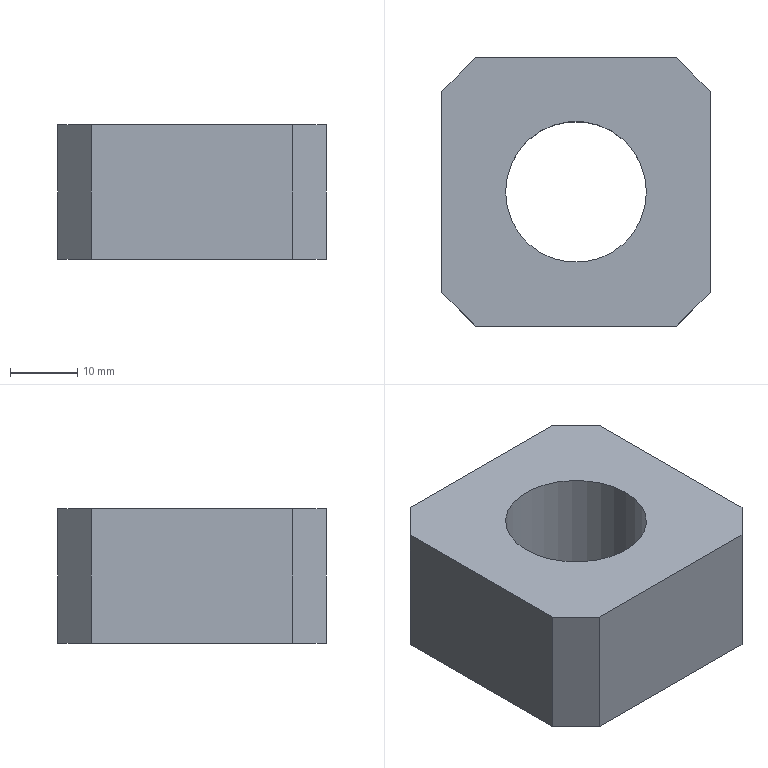CAM job | NX | 3-axis milling, drilling | part box 40 x 40 x 20 mm | stock box 45 x 45 x 25 mm
Tools:
number,name,description,diameter,corner_radius,flute_length,length,flutes
5,D10开粗,D10,10.0,0.0,25.0,75.0,2
7,D10精光,D10,10.0,0.0,25.0,75.0,2
2,D8倒角刀,DJ8-32,8.0,0.0,4.0,60.0,2
1,D50面刀,Milling Tool-5 Parameters,50.0,0.0,50.0,75.0,2
8,D15钻头,Drilling Tool,15.0,0.0,35.0,50.0,2
9,THREAD_MILL,Thread Mill,20.6,0.0,3.0,50.0,1
Operations:
program,operation,operation_type,tool,method,geometry_group,spindle_rpm,surface_speed,feed_per_tooth,feed_cut,feed_plunge,cut_length_mm,path_length_mm,cut_time_min,machine_time_min
XX-CNC1,PLANAR_MILL,PlanarMilling,D50面刀,METHOD,MCS_1,2000.0,314.0,0.2,800.0,100.0,114.0,169.8,0.1425,0.1481
XX-CNC1,PLANAR_MILL_COPY_1,PlanarMilling,D50面刀,METHOD,MCS_1,2000.0,314.0,0.2,800.0,100.0,114.0,170.0,0.1425,0.1481
XX-CNC1,DRILLING,Operation,D8倒角刀,METHOD,W1,2000.0,50.0,0.0375,150.0,0.0,4.5,69.0,0.03,0.0364
XX-CNC1,DRILLING_COPY,Operation,D15钻头,METHOD,W1,800.0,50.0,0.0375,40.0,0.0,31.0,122.0,0.775,0.7841
XX-CNC1,ADAPTIVE_MILLING,CavityMilling,D10开粗,METHOD,W1,3500.0,100.0,0.1178,1500.0,100.0,2473.274,2631.63,1.649,1.665
XX-CNC1,ADAPTIVE_MILLING_COPY,CavityMilling,D10开粗,METHOD,W1,3500.0,100.0,0.1178,1500.0,100.0,1757.21,1853.21,1.13,1.139
XX-CNC1,PLANAR_MILL_1_COPY_1,PlanarMilling,D10精光,METHOD,W1,2500.0,78.0,0.08,400.0,100.0,46.096,144.096,0.1152,0.125
XX-CNC1,PLANAR_MILL_1,PlanarMilling,D10精光,METHOD,W1,2500.0,62.0,0.12,600.0,100.0,379.142,580.368,0.6319,0.652
XX-CNC1,PLANAR_MILL_1_COPY,PlanarMilling,D8倒角刀,METHOD,W1,2500.0,62.0,0.12,600.0,100.0,173.757,234.757,0.2896,0.2957
XX-CNC1,PLANAR_MILL_1_COPY_COPY,PlanarMilling,D8倒角刀,METHOD,W1,3000.0,75.0,0.1,600.0,100.0,203.021,264.021,0.3384,0.3445
XX-CNC1,THREAD_MILLING,ThreadMilling,THREAD_MILL,METHOD,W1,2500.0,125.0,0.024,200.0,100.0,1421.909,1999.515,7.109,7.167
XX-CNC1,PLANAR_MILL_1_COPY_1_COPY,PlanarMilling,D10精光,METHOD,W1,2500.0,78.0,0.08,400.0,100.0,46.096,144.096,0.1152,0.125
XX-CNC1,PLANAR_MILL_1_COPY_COPY_COPY_1,PlanarMilling,D8倒角刀,METHOD,W1,3000.0,75.0,0.1,600.0,100.0,71.138,132.137,0.1186,0.1247
XX-CNC1,THREAD_MILLING_COPY,ThreadMilling,THREAD_MILL,METHOD,W1,2500.0,125.0,0.024,60.0,100.0,97.789,180.789,1.63,1.638
XX-CNC2,ADAPTIVE_MILLING_COPY_1,CavityMilling,D10开粗,METHOD,W1,3500.0,100.0,0.1178,1500.0,100.0,6790.747,6844.547,4.527,4.532
XX-CNC2,PLANAR_MILL_COPY,PlanarMilling,D50面刀,METHOD,MCS_1,2000.0,314.0,0.2,800.0,100.0,114.0,170.0,0.1425,0.1481
XX-CNC2,PLANAR_MILL_1_COPY_COPY_1,PlanarMilling,D8倒角刀,METHOD,W1,2500.0,62.0,0.12,600.0,100.0,173.757,234.757,0.2896,0.2957
XX-CNC2,PLANAR_MILL_1_COPY_COPY_COPY,PlanarMilling,D8倒角刀,METHOD,W1,3000.0,75.0,0.1,600.0,100.0,203.021,264.021,0.3384,0.3445